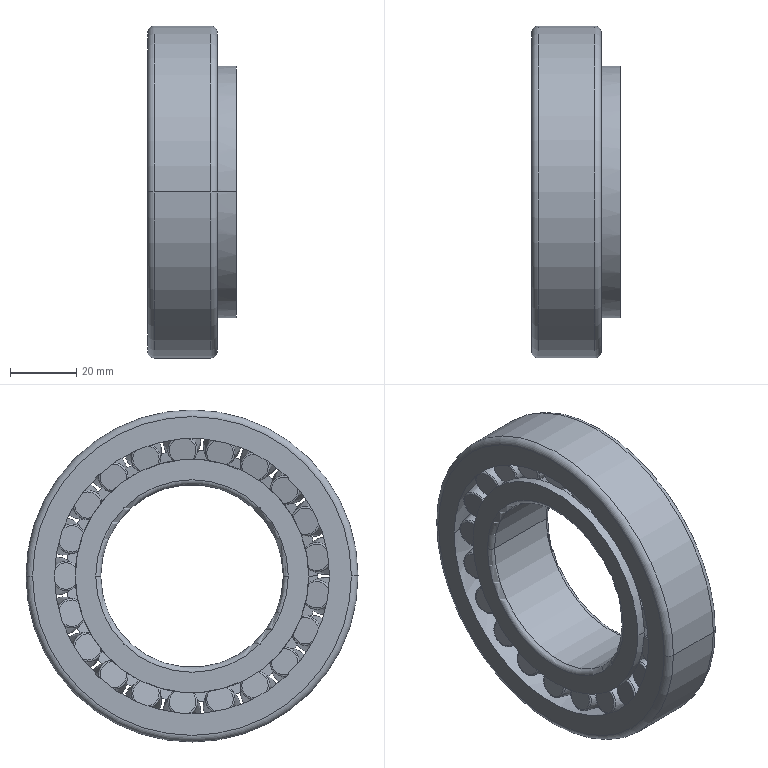Part | SolidWorks | features Revolution 3, CirPattern 1 | 1 solid | 196 faces | box 26.75 x 100 x 100 mm | volume 98923 mm3 | torus 92 | cone 50 | plane 46 | cylinder 8 | commonest cylinder face diameters 55 x2 70.308 x2 75.88 x2 100 x2